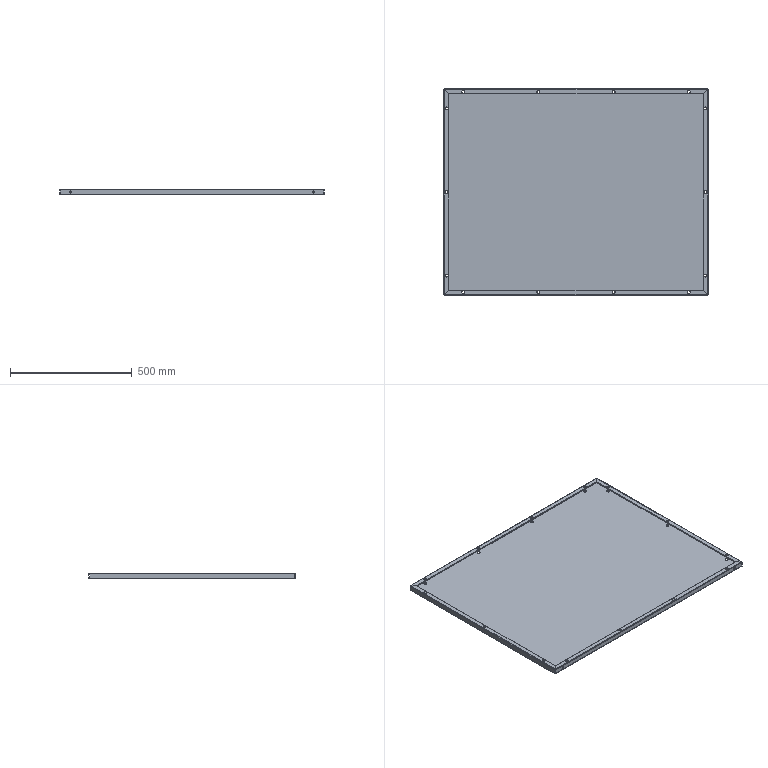Part | STEP file | 750078381 | 1 solid | 137 faces | box 1086 x 846 x 23 mm | volume 1590707 mm3 | cylinder 77 | plane 46 | spline 14 | commonest cylinder face diameters 12 x56 3 x8 6 x8 9 x4 2 x1